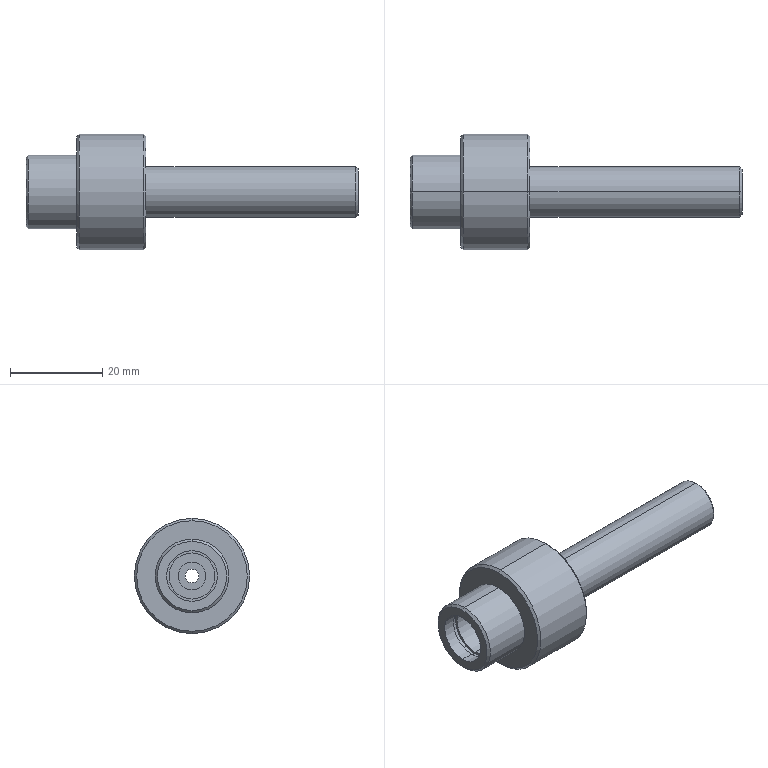Part | SolidWorks | features ICE 9, Chamfer 1, Extrusion 1, HoleWzd 1 | 1 solid | 41 faces | box 72 x 25 x 25 mm | volume 11483 mm3 | cylinder 22 | plane 11 | cone 8 | commonest cylinder face diameters 11 x6 3 x2 5.5 x2 6 x2 6.8 x2 10 x2
STEP:
#1=CARTESIAN_POINT('',(0.,0.,7.5));
#2=VERTEX_POINT('',#1);
#3=CARTESIAN_POINT('',(0.,0.,-7.5));
#4=VERTEX_POINT('',#3);
#5=CARTESIAN_POINT('',(0.,0.,0.));
#6=DIRECTION('',(-1.,0.,0.));
#7=DIRECTION('',(0.,0.,-1.));
#8=AXIS2_PLACEMENT_3D('',#5,#6,#7);
#9=CIRCLE('',#8,7.5);
#10=EDGE_CURVE('',#2,#4,#9,.T.);
#11=ORIENTED_EDGE('',*,*,#10,.F.);
#12=CARTESIAN_POINT('',(0.5,0.,8.));
#13=VERTEX_POINT('',#12);
#14=CARTESIAN_POINT('',(0.5,0.,8.));
#15=DIRECTION('',(0.7071,0.,0.7071));
#16=VECTOR('',#15,1000.);
#17=LINE('',#14,#16);
#18=EDGE_CURVE('',#2,#13,#17,.T.);
#19=ORIENTED_EDGE('',*,*,#18,.T.);
#20=CARTESIAN_POINT('',(0.5,0.,-8.));
#21=VERTEX_POINT('',#20);
#22=CARTESIAN_POINT('',(0.5,0.,0.));
#23=DIRECTION('',(1.,0.,0.));
#24=DIRECTION('',(0.,0.,-1.));
#25=AXIS2_PLACEMENT_3D('',#22,#23,#24);
#26=CIRCLE('',#25,8.);
#27=EDGE_CURVE('',#21,#13,#26,.T.);
#28=ORIENTED_EDGE('',*,*,#27,.F.);
#29=CARTESIAN_POINT('',(0.5,0.,-8.));
#30=DIRECTION('',(0.7071,0.,-0.7071));
#31=VECTOR('',#30,1000.);
#32=LINE('',#29,#31);
#33=EDGE_CURVE('',#4,#21,#32,.T.);
#34=ORIENTED_EDGE('',*,*,#33,.F.);
#35=EDGE_LOOP('',(#11,#19,#28,#34));
#36=FACE_OUTER_BOUND('',#35,.T.);
#37=CARTESIAN_POINT('',(0.5,0.,0.));
#38=DIRECTION('',(1.,0.,0.));
#39=DIRECTION('',(0.,0.,-1.));
#40=AXIS2_PLACEMENT_3D('',#37,#38,#39);
#41=CONICAL_SURFACE('',#40,8.,0.7854);
#42=ADVANCED_FACE('',(#36),#41,.T.);
#43=CARTESIAN_POINT('',(11.,0.,12.));
#44=VERTEX_POINT('',#43);
#45=CARTESIAN_POINT('',(11.,0.,-12.));
#46=VERTEX_POINT('',#45);
#47=CARTESIAN_POINT('',(11.,0.,0.));
#48=DIRECTION('',(-1.,0.,0.));
#49=DIRECTION('',(0.,0.,-1.));
#50=AXIS2_PLACEMENT_3D('',#47,#48,#49);
#51=CIRCLE('',#50,12.);
#52=EDGE_CURVE('',#44,#46,#51,.T.);
#53=ORIENTED_EDGE('',*,*,#52,.F.);
#54=CARTESIAN_POINT('',(11.5,0.,12.5));
#55=VERTEX_POINT('',#54);
#56=CARTESIAN_POINT('',(11.5,0.,12.5));
#57=DIRECTION('',(0.7071,0.,0.7071));
#58=VECTOR('',#57,1000.);
#59=LINE('',#56,#58);
#60=EDGE_CURVE('',#44,#55,#59,.T.);
#61=ORIENTED_EDGE('',*,*,#60,.T.);
#62=CARTESIAN_POINT('',(11.5,0.,-12.5));
#63=VERTEX_POINT('',#62);
#64=CARTESIAN_POINT('',(11.5,0.,0.));
#65=DIRECTION('',(1.,0.,0.));
#66=DIRECTION('',(0.,0.,-1.));
#67=AXIS2_PLACEMENT_3D('',#64,#65,#66);
#68=CIRCLE('',#67,12.5);
#69=EDGE_CURVE('',#63,#55,#68,.T.);
#70=ORIENTED_EDGE('',*,*,#69,.F.);
#71=CARTESIAN_POINT('',(11.5,0.,-12.5));
#72=DIRECTION('',(0.7071,0.,-0.7071));
#73=VECTOR('',#72,1000.);
#74=LINE('',#71,#73);
#75=EDGE_CURVE('',#46,#63,#74,.T.);
#76=ORIENTED_EDGE('',*,*,#75,.F.);
#77=EDGE_LOOP('',(#53,#61,#70,#76));
#78=FACE_OUTER_BOUND('',#77,.T.);
#79=CARTESIAN_POINT('',(11.5,0.,0.));
#80=DIRECTION('',(1.,0.,0.));
#81=DIRECTION('',(0.,0.,-1.));
#82=AXIS2_PLACEMENT_3D('',#79,#80,#81);
#83=CONICAL_SURFACE('',#82,12.5,0.7854);
#84=ADVANCED_FACE('',(#78),#83,.T.);
#85=CARTESIAN_POINT('',(26.,0.,-12.));
#86=VERTEX_POINT('',#85);
#87=CARTESIAN_POINT('',(26.,0.,12.));
#88=VERTEX_POINT('',#87);
#89=CARTESIAN_POINT('',(26.,0.,0.));
#90=DIRECTION('',(1.,0.,0.));
#91=DIRECTION('',(0.,0.,-1.));
#92=AXIS2_PLACEMENT_3D('',#89,#90,#91);
#93=CIRCLE('',#92,12.);
#94=EDGE_CURVE('',#86,#88,#93,.T.);
#95=ORIENTED_EDGE('',*,*,#94,.F.);
#96=CARTESIAN_POINT('',(25.5,0.,-12.5));
#97=VERTEX_POINT('',#96);
#98=CARTESIAN_POINT('',(26.,0.,-12.));
#99=DIRECTION('',(-0.7071,0.,-0.7071));
#100=VECTOR('',#99,1000.);
#101=LINE('',#98,#100);
#102=EDGE_CURVE('',#86,#97,#101,.T.);
#103=ORIENTED_EDGE('',*,*,#102,.T.);
#104=CARTESIAN_POINT('',(25.5,0.,12.5));
#105=VERTEX_POINT('',#104);
#106=CARTESIAN_POINT('',(25.5,0.,0.));
#107=DIRECTION('',(-1.,0.,0.));
#108=DIRECTION('',(0.,0.,-1.));
#109=AXIS2_PLACEMENT_3D('',#106,#107,#108);
#110=CIRCLE('',#109,12.5);
#111=EDGE_CURVE('',#105,#97,#110,.T.);
#112=ORIENTED_EDGE('',*,*,#111,.F.);
#113=CARTESIAN_POINT('',(26.,0.,12.));
#114=DIRECTION('',(-0.7071,0.,0.7071));
#115=VECTOR('',#114,1000.);
#116=LINE('',#113,#115);
#117=EDGE_CURVE('',#88,#105,#116,.T.);
#118=ORIENTED_EDGE('',*,*,#117,.F.);
#119=EDGE_LOOP('',(#95,#103,#112,#118));
#120=FACE_OUTER_BOUND('',#119,.T.);
#121=CARTESIAN_POINT('',(26.,0.,0.));
#122=DIRECTION('',(-1.,0.,0.));
#123=DIRECTION('',(0.,0.,1.));
#124=AXIS2_PLACEMENT_3D('',#121,#122,#123);
#125=CONICAL_SURFACE('',#124,12.,0.7854);
#126=ADVANCED_FACE('',(#120),#125,.T.);
#127=CARTESIAN_POINT('',(72.,0.,-5.));
#128=VERTEX_POINT('',#127);
#129=CARTESIAN_POINT('',(72.,0.,5.));
#130=VERTEX_POINT('',#129);
#131=CARTESIAN_POINT('',(72.,0.,0.));
#132=DIRECTION('',(1.,0.,0.));
#133=DIRECTION('',(0.,0.,-1.));
#134=AXIS2_PLACEMENT_3D('',#131,#132,#133);
#135=CIRCLE('',#134,5.);
#136=EDGE_CURVE('',#128,#130,#135,.T.);
#137=ORIENTED_EDGE('',*,*,#136,.F.);
#138=CARTESIAN_POINT('',(71.5,0.,-5.5));
#139=VERTEX_POINT('',#138);
#140=CARTESIAN_POINT('',(72.,0.,-5.));
#141=DIRECTION('',(-0.7071,0.,-0.7071));
#142=VECTOR('',#141,1000.);
#143=LINE('',#140,#142);
#144=EDGE_CURVE('',#128,#139,#143,.T.);
#145=ORIENTED_EDGE('',*,*,#144,.T.);
#146=CARTESIAN_POINT('',(71.5,0.,5.5));
#147=VERTEX_POINT('',#146);
#148=CARTESIAN_POINT('',(71.5,0.,0.));
#149=DIRECTION('',(-1.,0.,0.));
#150=DIRECTION('',(0.,0.,-1.));
#151=AXIS2_PLACEMENT_3D('',#148,#149,#150);
#152=CIRCLE('',#151,5.5);
#153=EDGE_CURVE('',#147,#139,#152,.T.);
#154=ORIENTED_EDGE('',*,*,#153,.F.);
#155=CARTESIAN_POINT('',(72.,0.,5.));
#156=DIRECTION('',(-0.7071,0.,0.7071));
#157=VECTOR('',#156,1000.);
#158=LINE('',#155,#157);
#159=EDGE_CURVE('',#130,#147,#158,.T.);
#160=ORIENTED_EDGE('',*,*,#159,.F.);
#161=EDGE_LOOP('',(#137,#145,#154,#160));
#162=FACE_OUTER_BOUND('',#161,.T.);
#163=CARTESIAN_POINT('',(72.,0.,0.));
#164=DIRECTION('',(-1.,0.,0.));
#165=DIRECTION('',(0.,0.,1.));
#166=AXIS2_PLACEMENT_3D('',#163,#164,#165);
#167=CONICAL_SURFACE('',#166,5.,0.7854);
#168=ADVANCED_FACE('',(#162),#167,.T.);
#169=CARTESIAN_POINT('',(29.,0.,-1.5));
#170=VERTEX_POINT('',#169);
#171=CARTESIAN_POINT('',(29.,0.,1.5));
#172=VERTEX_POINT('',#171);
#173=CARTESIAN_POINT('',(29.,0.,0.));
#174=DIRECTION('',(-1.,0.,0.));
#175=DIRECTION('',(0.,0.,1.));
#176=AXIS2_PLACEMENT_3D('',#173,#174,#175);
#177=CIRCLE('',#176,1.5);
#178=EDGE_CURVE('',#170,#172,#177,.T.);
#179=ORIENTED_EDGE('',*,*,#178,.T.);
#180=CARTESIAN_POINT('',(56.,0.,1.5));
#181=VERTEX_POINT('',#180);
#182=CARTESIAN_POINT('',(-32.,0.,1.5));
#183=DIRECTION('',(1.,0.,0.));
#184=VECTOR('',#183,1000.);
#185=LINE('',#182,#184);
#186=EDGE_CURVE('',#172,#181,#185,.T.);
#187=ORIENTED_EDGE('',*,*,#186,.T.);
#188=CARTESIAN_POINT('',(56.,0.,-1.5));
#189=VERTEX_POINT('',#188);
#190=CARTESIAN_POINT('',(56.,0.,0.));
#191=DIRECTION('',(1.,0.,0.));
#192=DIRECTION('',(0.,0.,-1.));
#193=AXIS2_PLACEMENT_3D('',#190,#191,#192);
#194=CIRCLE('',#193,1.5);
#195=EDGE_CURVE('',#181,#189,#194,.T.);
#196=ORIENTED_EDGE('',*,*,#195,.T.);
#197=CARTESIAN_POINT('',(-32.,0.,-1.5));
#198=DIRECTION('',(1.,0.,0.));
#199=VECTOR('',#198,1000.);
#200=LINE('',#197,#199);
#201=EDGE_CURVE('',#170,#189,#200,.T.);
#202=ORIENTED_EDGE('',*,*,#201,.F.);
#203=EDGE_LOOP('',(#179,#187,#196,#202));
#204=FACE_OUTER_BOUND('',#203,.T.);
#205=CARTESIAN_POINT('',(-32.,0.,0.));
#206=DIRECTION('',(1.,0.,0.));
#207=DIRECTION('',(0.,0.,-1.));
#208=AXIS2_PLACEMENT_3D('',#205,#206,#207);
#209=CYLINDRICAL_SURFACE('',#208,1.5);
#210=ADVANCED_FACE('',(#204),#209,.F.);
#211=CARTESIAN_POINT('',(56.,0.,2.75));
#212=VERTEX_POINT('',#211);
#213=CARTESIAN_POINT('',(56.,0.,-2.75));
#214=VERTEX_POINT('',#213);
#215=CARTESIAN_POINT('',(56.,0.,0.));
#216=DIRECTION('',(1.,0.,0.));
#217=DIRECTION('',(0.,0.,-1.));
#218=AXIS2_PLACEMENT_3D('',#215,#216,#217);
#219=CIRCLE('',#218,2.75);
#220=EDGE_CURVE('',#212,#214,#219,.T.);
#221=ORIENTED_EDGE('',*,*,#220,.F.);
#222=CARTESIAN_POINT('',(61.,0.,2.75));
#223=VERTEX_POINT('',#222);
#224=CARTESIAN_POINT('',(56.,0.,2.75));
#225=DIRECTION('',(1.,0.,0.));
#226=VECTOR('',#225,1000.);
#227=LINE('',#224,#226);
#228=EDGE_CURVE('',#212,#223,#227,.T.);
#229=ORIENTED_EDGE('',*,*,#228,.T.);
#230=CARTESIAN_POINT('',(61.,0.,-2.75));
#231=VERTEX_POINT('',#230);
#232=CARTESIAN_POINT('',(61.,0.,0.));
#233=DIRECTION('',(1.,0.,0.));
#234=DIRECTION('',(0.,0.,-1.));
#235=AXIS2_PLACEMENT_3D('',#232,#233,#234);
#236=CIRCLE('',#235,2.75);
#237=EDGE_CURVE('',#223,#231,#236,.T.);
#238=ORIENTED_EDGE('',*,*,#237,.T.);
#239=CARTESIAN_POINT('',(56.,0.,-2.75));
#240=DIRECTION('',(1.,0.,0.));
#241=VECTOR('',#240,1000.);
#242=LINE('',#239,#241);
#243=EDGE_CURVE('',#214,#231,#242,.T.);
#244=ORIENTED_EDGE('',*,*,#243,.F.);
#245=EDGE_LOOP('',(#221,#229,#238,#244));
#246=FACE_OUTER_BOUND('',#245,.T.);
#247=CARTESIAN_POINT('',(56.,0.,0.));
#248=DIRECTION('',(1.,0.,0.));
#249=DIRECTION('',(0.,0.,-1.));
#250=AXIS2_PLACEMENT_3D('',#247,#248,#249);
#251=CYLINDRICAL_SURFACE('',#250,2.75);
#252=ADVANCED_FACE('',(#246),#251,.F.);
#253=CARTESIAN_POINT('',(61.,0.,3.4));
#254=VERTEX_POINT('',#253);
#255=CARTESIAN_POINT('',(61.,0.,-3.4));
#256=VERTEX_POINT('',#255);
#257=CARTESIAN_POINT('',(61.,0.,0.));
#258=DIRECTION('',(1.,0.,0.));
#259=DIRECTION('',(0.,0.,-1.));
#260=AXIS2_PLACEMENT_3D('',#257,#258,#259);
#261=CIRCLE('',#260,3.4);
#262=EDGE_CURVE('',#254,#256,#261,.T.);
#263=ORIENTED_EDGE('',*,*,#262,.F.);
#264=CARTESIAN_POINT('',(72.,0.,3.4));
#265=VERTEX_POINT('',#264);
#266=CARTESIAN_POINT('',(72.,0.,3.4));
#267=DIRECTION('',(1.,0.,0.));
#268=VECTOR('',#267,1000.);
#269=LINE('',#266,#268);
#270=EDGE_CURVE('',#254,#265,#269,.T.);
#271=ORIENTED_EDGE('',*,*,#270,.T.);
#272=CARTESIAN_POINT('',(72.,0.,-3.4));
#273=VERTEX_POINT('',#272);
#274=CARTESIAN_POINT('',(72.,0.,0.));
#275=DIRECTION('',(1.,0.,0.));
#276=DIRECTION('',(0.,0.,-1.));
#277=AXIS2_PLACEMENT_3D('',#274,#275,#276);
#278=CIRCLE('',#277,3.4);
#279=EDGE_CURVE('',#265,#273,#278,.T.);
#280=ORIENTED_EDGE('',*,*,#279,.T.);
#281=CARTESIAN_POINT('',(72.,0.,-3.4));
#282=DIRECTION('',(1.,0.,0.));
#283=VECTOR('',#282,1000.);
#284=LINE('',#281,#283);
#285=EDGE_CURVE('',#256,#273,#284,.T.);
#286=ORIENTED_EDGE('',*,*,#285,.F.);
#287=EDGE_LOOP('',(#263,#271,#280,#286));
#288=FACE_OUTER_BOUND('',#287,.T.);
#289=CARTESIAN_POINT('',(72.,0.,0.));
#290=DIRECTION('',(1.,0.,0.));
#291=DIRECTION('',(0.,0.,-1.));
#292=AXIS2_PLACEMENT_3D('',#289,#290,#291);
#293=CYLINDRICAL_SURFACE('',#292,3.4);
#294=ADVANCED_FACE('',(#288),#293,.F.);
#295=CARTESIAN_POINT('',(29.,0.,-3.));
#296=VERTEX_POINT('',#295);
#297=CARTESIAN_POINT('',(29.,0.,3.));
#298=VERTEX_POINT('',#297);
#299=CARTESIAN_POINT('',(29.,0.,0.));
#300=DIRECTION('',(-1.,0.,0.));
#301=DIRECTION('',(0.,0.,1.));
#302=AXIS2_PLACEMENT_3D('',#299,#300,#301);
#303=CIRCLE('',#302,3.);
#304=EDGE_CURVE('',#296,#298,#303,.T.);
#305=ORIENTED_EDGE('',*,*,#304,.F.);
#306=CARTESIAN_POINT('',(14.,0.,-3.));
#307=VERTEX_POINT('',#306);
#308=CARTESIAN_POINT('',(29.,0.,-3.));
#309=DIRECTION('',(-1.,0.,0.));
#310=VECTOR('',#309,1000.);
#311=LINE('',#308,#310);
#312=EDGE_CURVE('',#296,#307,#311,.T.);
#313=ORIENTED_EDGE('',*,*,#312,.T.);
#314=CARTESIAN_POINT('',(14.,0.,3.));
#315=VERTEX_POINT('',#314);
#316=CARTESIAN_POINT('',(14.,0.,0.));
#317=DIRECTION('',(-1.,0.,0.));
#318=DIRECTION('',(0.,0.,1.));
#319=AXIS2_PLACEMENT_3D('',#316,#317,#318);
#320=CIRCLE('',#319,3.);
#321=EDGE_CURVE('',#307,#315,#320,.T.);
#322=ORIENTED_EDGE('',*,*,#321,.T.);
#323=CARTESIAN_POINT('',(29.,0.,3.));
#324=DIRECTION('',(-1.,0.,0.));
#325=VECTOR('',#324,1000.);
#326=LINE('',#323,#325);
#327=EDGE_CURVE('',#298,#315,#326,.T.);
#328=ORIENTED_EDGE('',*,*,#327,.F.);
#329=EDGE_LOOP('',(#305,#313,#322,#328));
#330=FACE_OUTER_BOUND('',#329,.T.);
#331=CARTESIAN_POINT('',(29.,0.,0.));
#332=DIRECTION('',(-1.,0.,0.));
#333=DIRECTION('',(0.,0.,1.));
#334=AXIS2_PLACEMENT_3D('',#331,#332,#333);
#335=CYLINDRICAL_SURFACE('',#334,3.);
#336=ADVANCED_FACE('',(#330),#335,.F.);
#337=CARTESIAN_POINT('',(14.,0.,-5.));
#338=VERTEX_POINT('',#337);
#339=CARTESIAN_POINT('',(14.,0.,5.));
#340=VERTEX_POINT('',#339);
#341=CARTESIAN_POINT('',(14.,0.,0.));
#342=DIRECTION('',(-1.,0.,0.));
#343=DIRECTION('',(0.,0.,1.));
#344=AXIS2_PLACEMENT_3D('',#341,#342,#343);
#345=CIRCLE('',#344,5.);
#346=EDGE_CURVE('',#338,#340,#345,.T.);
#347=ORIENTED_EDGE('',*,*,#346,.F.);
#348=CARTESIAN_POINT('',(11.,0.,-5.));
#349=VERTEX_POINT('',#348);
#350=CARTESIAN_POINT('',(14.,0.,-5.));
#351=DIRECTION('',(-1.,0.,0.));
#352=VECTOR('',#351,1000.);
#353=LINE('',#350,#352);
#354=EDGE_CURVE('',#338,#349,#353,.T.);
#355=ORIENTED_EDGE('',*,*,#354,.T.);
#356=CARTESIAN_POINT('',(11.,0.,5.));
#357=VERTEX_POINT('',#356);
#358=CARTESIAN_POINT('',(11.,0.,0.));
#359=DIRECTION('',(-1.,0.,0.));
#360=DIRECTION('',(0.,0.,1.));
#361=AXIS2_PLACEMENT_3D('',#358,#359,#360);
#362=CIRCLE('',#361,5.);
#363=EDGE_CURVE('',#349,#357,#362,.T.);
#364=ORIENTED_EDGE('',*,*,#363,.T.);
#365=CARTESIAN_POINT('',(14.,0.,5.));
#366=DIRECTION('',(-1.,0.,0.));
#367=VECTOR('',#366,1000.);
#368=LINE('',#365,#367);
#369=EDGE_CURVE('',#340,#357,#368,.T.);
#370=ORIENTED_EDGE('',*,*,#369,.F.);
#371=EDGE_LOOP('',(#347,#355,#364,#370));
#372=FACE_OUTER_BOUND('',#371,.T.);
#373=CARTESIAN_POINT('',(14.,0.,0.));
#374=DIRECTION('',(-1.,0.,0.));
#375=DIRECTION('',(0.,0.,1.));
#376=AXIS2_PLACEMENT_3D('',#373,#374,#375);
#377=CYLINDRICAL_SURFACE('',#376,5.);
#378=ADVANCED_FACE('',(#372),#377,.F.);
#379=CARTESIAN_POINT('',(11.,0.,-5.5));
#380=VERTEX_POINT('',#379);
#381=CARTESIAN_POINT('',(11.,0.,5.5));
#382=VERTEX_POINT('',#381);
#383=CARTESIAN_POINT('',(11.,0.,0.));
#384=DIRECTION('',(-1.,0.,0.));
#385=DIRECTION('',(0.,0.,1.));
#386=AXIS2_PLACEMENT_3D('',#383,#384,#385);
#387=CIRCLE('',#386,5.5);
#388=EDGE_CURVE('',#380,#382,#387,.T.);
#389=ORIENTED_EDGE('',*,*,#388,.F.);
#390=CARTESIAN_POINT('',(3.8,0.,-5.5));
#391=VERTEX_POINT('',#390);
#392=CARTESIAN_POINT('',(11.,0.,-5.5));
#393=DIRECTION('',(-1.,0.,0.));
#394=VECTOR('',#393,1000.);
#395=LINE('',#392,#394);
#396=EDGE_CURVE('',#380,#391,#395,.T.);
#397=ORIENTED_EDGE('',*,*,#396,.T.);
#398=CARTESIAN_POINT('',(3.8,0.,5.5));
#399=VERTEX_POINT('',#398);
#400=CARTESIAN_POINT('',(3.8,0.,0.));
#401=DIRECTION('',(1.,0.,0.));
#402=DIRECTION('',(0.,0.,1.));
#403=AXIS2_PLACEMENT_3D('',#400,#401,#402);
#404=CIRCLE('',#403,5.5);
#405=EDGE_CURVE('',#399,#391,#404,.T.);
#406=ORIENTED_EDGE('',*,*,#405,.F.);
#407=CARTESIAN_POINT('',(11.,0.,5.5));
#408=DIRECTION('',(-1.,0.,0.));
#409=VECTOR('',#408,1000.);
#410=LINE('',#407,#409);
#411=EDGE_CURVE('',#382,#399,#410,.T.);
#412=ORIENTED_EDGE('',*,*,#411,.F.);
#413=EDGE_LOOP('',(#389,#397,#406,#412));
#414=FACE_OUTER_BOUND('',#413,.T.);
#415=CARTESIAN_POINT('',(11.,0.,0.));
#416=DIRECTION('',(-1.,0.,0.));
#417=DIRECTION('',(0.,0.,1.));
#418=AXIS2_PLACEMENT_3D('',#415,#416,#417);
#419=CYLINDRICAL_SURFACE('',#418,5.5);
#420=ADVANCED_FACE('',(#414),#419,.F.);
#421=CARTESIAN_POINT('',(3.8,0.,-6.));
#422=VERTEX_POINT('',#421);
#423=CARTESIAN_POINT('',(3.8,0.,6.));
#424=VERTEX_POINT('',#423);
#425=CARTESIAN_POINT('',(3.8,0.,0.));
#426=DIRECTION('',(-1.,0.,0.));
#427=DIRECTION('',(0.,0.,1.));
#428=AXIS2_PLACEMENT_3D('',#425,#426,#427);
#429=CIRCLE('',#428,6.);
#430=EDGE_CURVE('',#422,#424,#429,.T.);
#431=ORIENTED_EDGE('',*,*,#430,.F.);
#432=CARTESIAN_POINT('',(2.7,0.,-6.));
#433=VERTEX_POINT('',#432);
#434=CARTESIAN_POINT('',(3.8,0.,-6.));
#435=DIRECTION('',(-1.,0.,0.));
#436=VECTOR('',#435,1000.);
#437=LINE('',#434,#436);
#438=EDGE_CURVE('',#422,#433,#437,.T.);
#439=ORIENTED_EDGE('',*,*,#438,.T.);
#440=CARTESIAN_POINT('',(2.7,0.,6.));
#441=VERTEX_POINT('',#440);
#442=CARTESIAN_POINT('',(2.7,0.,0.));
#443=DIRECTION('',(-1.,0.,0.));
#444=DIRECTION('',(0.,0.,1.));
#445=AXIS2_PLACEMENT_3D('',#442,#443,#444);
#446=CIRCLE('',#445,6.);
#447=EDGE_CURVE('',#433,#441,#446,.T.);
#448=ORIENTED_EDGE('',*,*,#447,.T.);
#449=CARTESIAN_POINT('',(3.8,0.,6.));
#450=DIRECTION('',(-1.,0.,0.));
#451=VECTOR('',#450,1000.);
#452=LINE('',#449,#451);
#453=EDGE_CURVE('',#424,#441,#452,.T.);
#454=ORIENTED_EDGE('',*,*,#453,.F.);
#455=EDGE_LOOP('',(#431,#439,#448,#454));
#456=FACE_OUTER_BOUND('',#455,.T.);
#457=CARTESIAN_POINT('',(3.8,0.,0.));
#458=DIRECTION('',(-1.,0.,0.));
#459=DIRECTION('',(0.,0.,1.));
#460=AXIS2_PLACEMENT_3D('',#457,#458,#459);
#461=CYLINDRICAL_SURFACE('',#460,6.);
#462=ADVANCED_FACE('',(#456),#461,.F.);
#463=CARTESIAN_POINT('',(2.7,0.,5.5));
#464=VERTEX_POINT('',#463);
#465=CARTESIAN_POINT('',(2.7,0.,-5.5));
#466=VERTEX_POINT('',#465);
#467=CARTESIAN_POINT('',(2.7,0.,0.));
#468=DIRECTION('',(1.,0.,0.));
#469=DIRECTION('',(0.,0.,1.));
#470=AXIS2_PLACEMENT_3D('',#467,#468,#469);
#471=CIRCLE('',#470,5.5);
#472=EDGE_CURVE('',#464,#466,#471,.T.);
#473=ORIENTED_EDGE('',*,*,#472,.T.);
#474=CARTESIAN_POINT('',(0.,0.,-5.5));
#475=VERTEX_POINT('',#474);
#476=CARTESIAN_POINT('',(11.,0.,-5.5));
#477=DIRECTION('',(-1.,0.,0.));
#478=VECTOR('',#477,1000.);
#479=LINE('',#476,#478);
#480=EDGE_CURVE('',#466,#475,#479,.T.);
#481=ORIENTED_EDGE('',*,*,#480,.T.);
#482=CARTESIAN_POINT('',(0.,0.,5.5));
#483=VERTEX_POINT('',#482);
#484=CARTESIAN_POINT('',(0.,0.,0.));
#485=DIRECTION('',(-1.,0.,0.));
#486=DIRECTION('',(0.,0.,1.));
#487=AXIS2_PLACEMENT_3D('',#484,#485,#486);
#488=CIRCLE('',#487,5.5);
#489=EDGE_CURVE('',#475,#483,#488,.T.);
#490=ORIENTED_EDGE('',*,*,#489,.T.);
#491=CARTESIAN_POINT('',(11.,0.,5.5));
#492=DIRECTION('',(-1.,0.,0.));
#493=VECTOR('',#492,1000.);
#494=LINE('',#491,#493);
#495=EDGE_CURVE('',#464,#483,#494,.T.);
#496=ORIENTED_EDGE('',*,*,#495,.F.);
#497=EDGE_LOOP('',(#473,#481,#490,#496));
#498=FACE_OUTER_BOUND('',#497,.T.);
#499=CARTESIAN_POINT('',(11.,0.,0.));
#500=DIRECTION('',(-1.,0.,0.));
#501=DIRECTION('',(0.,0.,1.));
#502=AXIS2_PLACEMENT_3D('',#499,#500,#501);
#503=CYLINDRICAL_SURFACE('',#502,5.5);
#504=ADVANCED_FACE('',(#498),#503,.F.);
#505=ORIENTED_EDGE('',*,*,#153,.T.);
#506=CARTESIAN_POINT('',(26.,0.,-5.5));
#507=VERTEX_POINT('',#506);
#508=CARTESIAN_POINT('',(72.,0.,-5.5));
#509=DIRECTION('',(-1.,0.,0.));
#510=VECTOR('',#509,1000.);
#511=LINE('',#508,#510);
#512=EDGE_CURVE('',#139,#507,#511,.T.);
#513=ORIENTED_EDGE('',*,*,#512,.T.);
#514=CARTESIAN_POINT('',(26.,0.,5.5));
#515=VERTEX_POINT('',#514);
#516=CARTESIAN_POINT('',(26.,0.,0.));
#517=DIRECTION('',(1.,0.,0.));
#518=DIRECTION('',(0.,0.,-1.));
#519=AXIS2_PLACEMENT_3D('',#516,#517,#518);
#520=CIRCLE('',#519,5.5);
#521=EDGE_CURVE('',#507,#515,#520,.T.);
#522=ORIENTED_EDGE('',*,*,#521,.T.);
#523=CARTESIAN_POINT('',(72.,0.,5.5));
#524=DIRECTION('',(-1.,0.,0.));
#525=VECTOR('',#524,1000.);
#526=LINE('',#523,#525);
#527=EDGE_CURVE('',#147,#515,#526,.T.);
#528=ORIENTED_EDGE('',*,*,#527,.F.);
#529=EDGE_LOOP('',(#505,#513,#522,#528));
#530=FACE_OUTER_BOUND('',#529,.T.);
#531=CARTESIAN_POINT('',(72.,0.,0.));
#532=DIRECTION('',(-1.,0.,0.));
#533=DIRECTION('',(0.,0.,1.));
#534=AXIS2_PLACEMENT_3D('',#531,#532,#533);
#535=CYLINDRICAL_SURFACE('',#534,5.5);
#536=ADVANCED_FACE('',(#530),#535,.T.);
#537=ORIENTED_EDGE('',*,*,#111,.T.);
#538=CARTESIAN_POINT('',(26.,0.,-12.5));
#539=DIRECTION('',(-1.,0.,0.));
#540=VECTOR('',#539,1000.);
#541=LINE('',#538,#540);
#542=EDGE_CURVE('',#97,#63,#541,.T.);
#543=ORIENTED_EDGE('',*,*,#542,.T.);
#544=ORIENTED_EDGE('',*,*,#69,.T.);
#545=CARTESIAN_POINT('',(26.,0.,12.5));
#546=DIRECTION('',(-1.,0.,0.));
#547=VECTOR('',#546,1000.);
#548=LINE('',#545,#547);
#549=EDGE_CURVE('',#105,#55,#548,.T.);
#550=ORIENTED_EDGE('',*,*,#549,.F.);
#551=EDGE_LOOP('',(#537,#543,#544,#550));
#552=FACE_OUTER_BOUND('',#551,.T.);
#553=CARTESIAN_POINT('',(26.,0.,0.));
#554=DIRECTION('',(-1.,0.,0.));
#555=DIRECTION('',(0.,0.,1.));
#556=AXIS2_PLACEMENT_3D('',#553,#554,#555);
#557=CYLINDRICAL_SURFACE('',#556,12.5);
#558=ADVANCED_FACE('',(#552),#557,.T.);
#559=CARTESIAN_POINT('',(11.,0.,-8.));
#560=VERTEX_POINT('',#559);
#561=CARTESIAN_POINT('',(11.,0.,8.));
#562=VERTEX_POINT('',#561);
#563=CARTESIAN_POINT('',(11.,0.,0.));
#564=DIRECTION('',(1.,0.,0.));
#565=DIRECTION('',(0.,0.,-1.));
#566=AXIS2_PLACEMENT_3D('',#563,#564,#565);
#567=CIRCLE('',#566,8.);
#568=EDGE_CURVE('',#560,#562,#567,.T.);
#569=ORIENTED_EDGE('',*,*,#568,.F.);
#570=CARTESIAN_POINT('',(11.,0.,-8.));
#571=DIRECTION('',(-1.,0.,0.));
#572=VECTOR('',#571,1000.);
#573=LINE('',#570,#572);
#574=EDGE_CURVE('',#560,#21,#573,.T.);
#575=ORIENTED_EDGE('',*,*,#574,.T.);
#576=ORIENTED_EDGE('',*,*,#27,.T.);
#577=CARTESIAN_POINT('',(11.,0.,8.));
#578=DIRECTION('',(-1.,0.,0.));
#579=VECTOR('',#578,1000.);
#580=LINE('',#577,#579);
#581=EDGE_CURVE('',#562,#13,#580,.T.);
#582=ORIENTED_EDGE('',*,*,#581,.F.);
#583=EDGE_LOOP('',(#569,#575,#576,#582));
#584=FACE_OUTER_BOUND('',#583,.T.);
#585=CARTESIAN_POINT('',(11.,0.,0.));
#586=DIRECTION('',(-1.,0.,0.));
#587=DIRECTION('',(0.,0.,1.));
#588=AXIS2_PLACEMENT_3D('',#585,#586,#587);
#589=CYLINDRICAL_SURFACE('',#588,8.);
#590=ADVANCED_FACE('',(#584),#589,.T.);
#591=ORIENTED_EDGE('',*,*,#574,.F.);
#592=CARTESIAN_POINT('',(11.,0.,0.));
#593=DIRECTION('',(1.,0.,0.));
#594=DIRECTION('',(0.,0.,-1.));
#595=AXIS2_PLACEMENT_3D('',#592,#593,#594);
#596=CIRCLE('',#595,8.);
#597=EDGE_CURVE('',#562,#560,#596,.T.);
#598=ORIENTED_EDGE('',*,*,#597,.F.);
#599=ORIENTED_EDGE('',*,*,#581,.T.);
#600=CARTESIAN_POINT('',(0.5,0.,0.));
#601=DIRECTION('',(1.,0.,0.));
#602=DIRECTION('',(0.,0.,-1.));
#603=AXIS2_PLACEMENT_3D('',#600,#601,#602);
#604=CIRCLE('',#603,8.);
#605=EDGE_CURVE('',#13,#21,#604,.T.);
#606=ORIENTED_EDGE('',*,*,#605,.T.);
#607=EDGE_LOOP('',(#591,#598,#599,#606));
#608=FACE_OUTER_BOUND('',#607,.T.);
#609=CARTESIAN_POINT('',(11.,0.,0.));
#610=DIRECTION('',(-1.,0.,0.));
#611=DIRECTION('',(0.,0.,1.));
#612=AXIS2_PLACEMENT_3D('',#609,#610,#611);
#613=CYLINDRICAL_SURFACE('',#612,8.);
#614=ADVANCED_FACE('',(#608),#613,.T.);
#615=CARTESIAN_POINT('',(0.,0.,0.));
#616=DIRECTION('',(-1.,0.,0.));
#617=DIRECTION('',(0.,0.,-1.));
#618=AXIS2_PLACEMENT_3D('',#615,#616,#617);
#619=CIRCLE('',#618,7.5);
#620=EDGE_CURVE('',#4,#2,#619,.T.);
#621=ORIENTED_EDGE('',*,*,#620,.T.);
#622=ORIENTED_EDGE('',*,*,#10,.T.);
#623=EDGE_LOOP('',(#621,#622));
#624=FACE_OUTER_BOUND('',#623,.T.);
#625=CARTESIAN_POINT('',(0.,0.,0.));
#626=DIRECTION('',(-1.,0.,0.));
#627=DIRECTION('',(0.,0.,1.));
#628=AXIS2_PLACEMENT_3D('',#625,#626,#627);
#629=CIRCLE('',#628,5.5);
#630=EDGE_CURVE('',#483,#475,#629,.T.);
#631=ORIENTED_EDGE('',*,*,#630,.F.);
#632=ORIENTED_EDGE('',*,*,#489,.F.);
#633=EDGE_LOOP('',(#631,#632));
#634=FACE_BOUND('',#633,.T.);
#635=CARTESIAN_POINT('',(0.,0.,0.));
#636=DIRECTION('',(1.,0.,0.));
#637=DIRECTION('',(0.,0.,-1.));
#638=AXIS2_PLACEMENT_3D('',#635,#636,#637);
#639=PLANE('',#638);
#640=ADVANCED_FACE('',(#624,#634),#639,.F.);
#641=ORIENTED_EDGE('',*,*,#542,.F.);
#642=CARTESIAN_POINT('',(25.5,0.,0.));
#643=DIRECTION('',(-1.,0.,0.));
#644=DIRECTION('',(0.,0.,-1.));
#645=AXIS2_PLACEMENT_3D('',#642,#643,#644);
#646=CIRCLE('',#645,12.5);
#647=EDGE_CURVE('',#97,#105,#646,.T.);
#648=ORIENTED_EDGE('',*,*,#647,.T.);
#649=ORIENTED_EDGE('',*,*,#549,.T.);
#650=CARTESIAN_POINT('',(11.5,0.,0.));
#651=DIRECTION('',(1.,0.,0.));
#652=DIRECTION('',(0.,0.,-1.));
#653=AXIS2_PLACEMENT_3D('',#650,#651,#652);
#654=CIRCLE('',#653,12.5);
#655=EDGE_CURVE('',#55,#63,#654,.T.);
#656=ORIENTED_EDGE('',*,*,#655,.T.);
#657=EDGE_LOOP('',(#641,#648,#649,#656));
#658=FACE_OUTER_BOUND('',#657,.T.);
#659=CARTESIAN_POINT('',(26.,0.,0.));
#660=DIRECTION('',(-1.,0.,0.));
#661=DIRECTION('',(0.,0.,1.));
#662=AXIS2_PLACEMENT_3D('',#659,#660,#661);
#663=CYLINDRICAL_SURFACE('',#662,12.5);
#664=ADVANCED_FACE('',(#658),#663,.T.);
#665=CARTESIAN_POINT('',(26.,0.,0.));
#666=DIRECTION('',(1.,0.,0.));
#667=DIRECTION('',(0.,0.,-1.));
#668=AXIS2_PLACEMENT_3D('',#665,#666,#667);
#669=CIRCLE('',#668,12.);
#670=EDGE_CURVE('',#88,#86,#669,.T.);
#671=ORIENTED_EDGE('',*,*,#670,.T.);
#672=ORIENTED_EDGE('',*,*,#94,.T.);
#673=EDGE_LOOP('',(#671,#672));
#674=FACE_OUTER_BOUND('',#673,.T.);
#675=CARTESIAN_POINT('',(26.,0.,0.));
#676=DIRECTION('',(1.,0.,0.));
#677=DIRECTION('',(0.,0.,-1.));
#678=AXIS2_PLACEMENT_3D('',#675,#676,#677);
#679=CIRCLE('',#678,5.5);
#680=EDGE_CURVE('',#515,#507,#679,.T.);
#681=ORIENTED_EDGE('',*,*,#680,.F.);
#682=ORIENTED_EDGE('',*,*,#521,.F.);
#683=EDGE_LOOP('',(#681,#682));
#684=FACE_BOUND('',#683,.T.);
#685=CARTESIAN_POINT('',(26.,0.,0.));
#686=DIRECTION('',(1.,0.,0.));
#687=DIRECTION('',(0.,0.,-1.));
#688=AXIS2_PLACEMENT_3D('',#685,#686,#687);
#689=PLANE('',#688);
#690=ADVANCED_FACE('',(#674,#684),#689,.T.);
#691=CARTESIAN_POINT('',(11.,0.,0.));
#692=DIRECTION('',(-1.,0.,0.));
#693=DIRECTION('',(0.,0.,-1.));
#694=AXIS2_PLACEMENT_3D('',#691,#692,#693);
#695=CIRCLE('',#694,12.);
#696=EDGE_CURVE('',#46,#44,#695,.T.);
#697=ORIENTED_EDGE('',*,*,#696,.T.);
#698=ORIENTED_EDGE('',*,*,#52,.T.);
#699=EDGE_LOOP('',(#697,#698));
#700=FACE_OUTER_BOUND('',#699,.T.);
#701=ORIENTED_EDGE('',*,*,#597,.T.);
#702=ORIENTED_EDGE('',*,*,#568,.T.);
#703=EDGE_LOOP('',(#701,#702));
#704=FACE_BOUND('',#703,.T.);
#705=CARTESIAN_POINT('',(11.,0.,0.));
#706=DIRECTION('',(1.,0.,0.));
#707=DIRECTION('',(0.,0.,-1.));
#708=AXIS2_PLACEMENT_3D('',#705,#706,#707);
#709=PLANE('',#708);
#710=ADVANCED_FACE('',(#700,#704),#709,.F.);
#711=ORIENTED_EDGE('',*,*,#512,.F.);
#712=CARTESIAN_POINT('',(71.5,0.,0.));
#713=DIRECTION('',(-1.,0.,0.));
#714=DIRECTION('',(0.,0.,-1.));
#715=AXIS2_PLACEMENT_3D('',#712,#713,#714);
#716=CIRCLE('',#715,5.5);
#717=EDGE_CURVE('',#139,#147,#716,.T.);
#718=ORIENTED_EDGE('',*,*,#717,.T.);
#719=ORIENTED_EDGE('',*,*,#527,.T.);
#720=ORIENTED_EDGE('',*,*,#680,.T.);
#721=EDGE_LOOP('',(#711,#718,#719,#720));
#722=FACE_OUTER_BOUND('',#721,.T.);
#723=CARTESIAN_POINT('',(72.,0.,0.));
#724=DIRECTION('',(-1.,0.,0.));
#725=DIRECTION('',(0.,0.,1.));
#726=AXIS2_PLACEMENT_3D('',#723,#724,#725);
#727=CYLINDRICAL_SURFACE('',#726,5.5);
#728=ADVANCED_FACE('',(#722),#727,.T.);
#729=CARTESIAN_POINT('',(72.,0.,0.));
#730=DIRECTION('',(1.,0.,0.));
#731=DIRECTION('',(0.,0.,-1.));
#732=AXIS2_PLACEMENT_3D('',#729,#730,#731);
#733=CIRCLE('',#732,5.);
#734=EDGE_CURVE('',#130,#128,#733,.T.);
#735=ORIENTED_EDGE('',*,*,#734,.T.);
#736=ORIENTED_EDGE('',*,*,#136,.T.);
#737=EDGE_LOOP('',(#735,#736));
#738=FACE_OUTER_BOUND('',#737,.T.);
#739=CARTESIAN_POINT('',(72.,0.,0.));
#740=DIRECTION('',(1.,0.,0.));
#741=DIRECTION('',(0.,0.,-1.));
#742=AXIS2_PLACEMENT_3D('',#739,#740,#741);
#743=CIRCLE('',#742,3.4);
#744=EDGE_CURVE('',#273,#265,#743,.T.);
#745=ORIENTED_EDGE('',*,*,#744,.F.);
#746=ORIENTED_EDGE('',*,*,#279,.F.);
#747=EDGE_LOOP('',(#745,#746));
#748=FACE_BOUND('',#747,.T.);
#749=CARTESIAN_POINT('',(72.,0.,0.));
#750=DIRECTION('',(1.,0.,0.));
#751=DIRECTION('',(0.,0.,-1.));
#752=AXIS2_PLACEMENT_3D('',#749,#750,#751);
#753=PLANE('',#752);
#754=ADVANCED_FACE('',(#738,#748),#753,.T.);
#755=ORIENTED_EDGE('',*,*,#480,.F.);
#756=CARTESIAN_POINT('',(2.7,0.,0.));
#757=DIRECTION('',(1.,0.,0.));
#758=DIRECTION('',(0.,0.,1.));
#759=AXIS2_PLACEMENT_3D('',#756,#757,#758);
#760=CIRCLE('',#759,5.5);
#761=EDGE_CURVE('',#466,#464,#760,.T.);
#762=ORIENTED_EDGE('',*,*,#761,.T.);
#763=ORIENTED_EDGE('',*,*,#495,.T.);
#764=ORIENTED_EDGE('',*,*,#630,.T.);
#765=EDGE_LOOP('',(#755,#762,#763,#764));
#766=FACE_OUTER_BOUND('',#765,.T.);
#767=CARTESIAN_POINT('',(11.,0.,0.));
#768=DIRECTION('',(-1.,0.,0.));
#769=DIRECTION('',(0.,0.,1.));
#770=AXIS2_PLACEMENT_3D('',#767,#768,#769);
#771=CYLINDRICAL_SURFACE('',#770,5.5);
#772=ADVANCED_FACE('',(#766),#771,.F.);
#773=CARTESIAN_POINT('',(3.8,0.,0.));
#774=DIRECTION('',(-1.,0.,0.));
#775=DIRECTION('',(0.,0.,1.));
#776=AXIS2_PLACEMENT_3D('',#773,#774,#775);
#777=CIRCLE('',#776,6.);
#778=EDGE_CURVE('',#424,#422,#777,.T.);
#779=ORIENTED_EDGE('',*,*,#778,.T.);
#780=ORIENTED_EDGE('',*,*,#430,.T.);
#781=EDGE_LOOP('',(#779,#780));
#782=FACE_OUTER_BOUND('',#781,.T.);
#783=ORIENTED_EDGE('',*,*,#405,.T.);
#784=CARTESIAN_POINT('',(3.8,0.,0.));
#785=DIRECTION('',(1.,0.,0.));
#786=DIRECTION('',(0.,0.,1.));
#787=AXIS2_PLACEMENT_3D('',#784,#785,#786);
#788=CIRCLE('',#787,5.5);
#789=EDGE_CURVE('',#391,#399,#788,.T.);
#790=ORIENTED_EDGE('',*,*,#789,.T.);
#791=EDGE_LOOP('',(#783,#790));
#792=FACE_BOUND('',#791,.T.);
#793=CARTESIAN_POINT('',(3.8,0.,0.));
#794=DIRECTION('',(-1.,0.,0.));
#795=DIRECTION('',(0.,0.,1.));
#796=AXIS2_PLACEMENT_3D('',#793,#794,#795);
#797=PLANE('',#796);
#798=ADVANCED_FACE('',(#782,#792),#797,.T.);
#799=CARTESIAN_POINT('',(2.7,0.,0.));
#800=DIRECTION('',(-1.,0.,0.));
#801=DIRECTION('',(0.,0.,1.));
#802=AXIS2_PLACEMENT_3D('',#799,#800,#801);
#803=CIRCLE('',#802,6.);
#804=EDGE_CURVE('',#441,#433,#803,.T.);
#805=ORIENTED_EDGE('',*,*,#804,.F.);
#806=ORIENTED_EDGE('',*,*,#447,.F.);
#807=EDGE_LOOP('',(#805,#806));
#808=FACE_OUTER_BOUND('',#807,.T.);
#809=ORIENTED_EDGE('',*,*,#472,.F.);
#810=ORIENTED_EDGE('',*,*,#761,.F.);
#811=EDGE_LOOP('',(#809,#810));
#812=FACE_BOUND('',#811,.T.);
#813=CARTESIAN_POINT('',(2.7,0.,0.));
#814=DIRECTION('',(-1.,0.,0.));
#815=DIRECTION('',(0.,0.,1.));
#816=AXIS2_PLACEMENT_3D('',#813,#814,#815);
#817=PLANE('',#816);
#818=ADVANCED_FACE('',(#808,#812),#817,.F.);
#819=ORIENTED_EDGE('',*,*,#438,.F.);
#820=ORIENTED_EDGE('',*,*,#778,.F.);
#821=ORIENTED_EDGE('',*,*,#453,.T.);
#822=ORIENTED_EDGE('',*,*,#804,.T.);
#823=EDGE_LOOP('',(#819,#820,#821,#822));
#824=FACE_OUTER_BOUND('',#823,.T.);
#825=CARTESIAN_POINT('',(3.8,0.,0.));
#826=DIRECTION('',(-1.,0.,0.));
#827=DIRECTION('',(0.,0.,1.));
#828=AXIS2_PLACEMENT_3D('',#825,#826,#827);
#829=CYLINDRICAL_SURFACE('',#828,6.);
#830=ADVANCED_FACE('',(#824),#829,.F.);
#831=CARTESIAN_POINT('',(11.,0.,0.));
#832=DIRECTION('',(-1.,0.,0.));
#833=DIRECTION('',(0.,0.,1.));
#834=AXIS2_PLACEMENT_3D('',#831,#832,#833);
#835=CIRCLE('',#834,5.);
#836=EDGE_CURVE('',#357,#349,#835,.T.);
#837=ORIENTED_EDGE('',*,*,#836,.F.);
#838=ORIENTED_EDGE('',*,*,#363,.F.);
#839=EDGE_LOOP('',(#837,#838));
#840=FACE_BOUND('',#839,.T.);
#841=CARTESIAN_POINT('',(11.,0.,0.));
#842=DIRECTION('',(-1.,0.,0.));
#843=DIRECTION('',(0.,0.,1.));
#844=AXIS2_PLACEMENT_3D('',#841,#842,#843);
#845=CIRCLE('',#844,5.5);
#846=EDGE_CURVE('',#382,#380,#845,.T.);
#847=ORIENTED_EDGE('',*,*,#846,.T.);
#848=ORIENTED_EDGE('',*,*,#388,.T.);
#849=EDGE_LOOP('',(#847,#848));
#850=FACE_OUTER_BOUND('',#849,.T.);
#851=CARTESIAN_POINT('',(11.,0.,0.));
#852=DIRECTION('',(-1.,0.,0.));
#853=DIRECTION('',(0.,0.,1.));
#854=AXIS2_PLACEMENT_3D('',#851,#852,#853);
#855=PLANE('',#854);
#856=ADVANCED_FACE('',(#840,#850),#855,.T.);
#857=ORIENTED_EDGE('',*,*,#396,.F.);
#858=ORIENTED_EDGE('',*,*,#846,.F.);
#859=ORIENTED_EDGE('',*,*,#411,.T.);
#860=ORIENTED_EDGE('',*,*,#789,.F.);
#861=EDGE_LOOP('',(#857,#858,#859,#860));
#862=FACE_OUTER_BOUND('',#861,.T.);
#863=CARTESIAN_POINT('',(11.,0.,0.));
#864=DIRECTION('',(-1.,0.,0.));
#865=DIRECTION('',(0.,0.,1.));
#866=AXIS2_PLACEMENT_3D('',#863,#864,#865);
#867=CYLINDRICAL_SURFACE('',#866,5.5);
#868=ADVANCED_FACE('',(#862),#867,.F.);
#869=ORIENTED_EDGE('',*,*,#354,.F.);
#870=CARTESIAN_POINT('',(14.,0.,0.));
#871=DIRECTION('',(-1.,0.,0.));
#872=DIRECTION('',(0.,0.,1.));
#873=AXIS2_PLACEMENT_3D('',#870,#871,#872);
#874=CIRCLE('',#873,5.);
#875=EDGE_CURVE('',#340,#338,#874,.T.);
#876=ORIENTED_EDGE('',*,*,#875,.F.);
#877=ORIENTED_EDGE('',*,*,#369,.T.);
#878=ORIENTED_EDGE('',*,*,#836,.T.);
#879=EDGE_LOOP('',(#869,#876,#877,#878));
#880=FACE_OUTER_BOUND('',#879,.T.);
#881=CARTESIAN_POINT('',(14.,0.,0.));
#882=DIRECTION('',(-1.,0.,0.));
#883=DIRECTION('',(0.,0.,1.));
#884=AXIS2_PLACEMENT_3D('',#881,#882,#883);
#885=CYLINDRICAL_SURFACE('',#884,5.);
#886=ADVANCED_FACE('',(#880),#885,.F.);
#887=CARTESIAN_POINT('',(14.,0.,0.));
#888=DIRECTION('',(-1.,0.,0.));
#889=DIRECTION('',(0.,0.,1.));
#890=AXIS2_PLACEMENT_3D('',#887,#888,#889);
#891=CIRCLE('',#890,3.);
#892=EDGE_CURVE('',#315,#307,#891,.T.);
#893=ORIENTED_EDGE('',*,*,#892,.F.);
#894=ORIENTED_EDGE('',*,*,#321,.F.);
#895=EDGE_LOOP('',(#893,#894));
#896=FACE_BOUND('',#895,.T.);
#897=ORIENTED_EDGE('',*,*,#875,.T.);
#898=ORIENTED_EDGE('',*,*,#346,.T.);
#899=EDGE_LOOP('',(#897,#898));
#900=FACE_OUTER_BOUND('',#899,.T.);
#901=CARTESIAN_POINT('',(14.,0.,0.));
#902=DIRECTION('',(-1.,0.,0.));
#903=DIRECTION('',(0.,0.,1.));
#904=AXIS2_PLACEMENT_3D('',#901,#902,#903);
#905=PLANE('',#904);
#906=ADVANCED_FACE('',(#896,#900),#905,.T.);
#907=ORIENTED_EDGE('',*,*,#312,.F.);
#908=CARTESIAN_POINT('',(29.,0.,0.));
#909=DIRECTION('',(-1.,0.,0.));
#910=DIRECTION('',(0.,0.,1.));
#911=AXIS2_PLACEMENT_3D('',#908,#909,#910);
#912=CIRCLE('',#911,3.);
#913=EDGE_CURVE('',#298,#296,#912,.T.);
#914=ORIENTED_EDGE('',*,*,#913,.F.);
#915=ORIENTED_EDGE('',*,*,#327,.T.);
#916=ORIENTED_EDGE('',*,*,#892,.T.);
#917=EDGE_LOOP('',(#907,#914,#915,#916));
#918=FACE_OUTER_BOUND('',#917,.T.);
#919=CARTESIAN_POINT('',(29.,0.,0.));
#920=DIRECTION('',(-1.,0.,0.));
#921=DIRECTION('',(0.,0.,1.));
#922=AXIS2_PLACEMENT_3D('',#919,#920,#921);
#923=CYLINDRICAL_SURFACE('',#922,3.);
#924=ADVANCED_FACE('',(#918),#923,.F.);
#925=ORIENTED_EDGE('',*,*,#178,.F.);
#926=CARTESIAN_POINT('',(29.,0.,0.));
#927=DIRECTION('',(-1.,0.,0.));
#928=DIRECTION('',(0.,0.,1.));
#929=AXIS2_PLACEMENT_3D('',#926,#927,#928);
#930=CIRCLE('',#929,1.5);
#931=EDGE_CURVE('',#172,#170,#930,.T.);
#932=ORIENTED_EDGE('',*,*,#931,.F.);
#933=EDGE_LOOP('',(#925,#932));
#934=FACE_BOUND('',#933,.T.);
#935=ORIENTED_EDGE('',*,*,#913,.T.);
#936=ORIENTED_EDGE('',*,*,#304,.T.);
#937=EDGE_LOOP('',(#935,#936));
#938=FACE_OUTER_BOUND('',#937,.T.);
#939=CARTESIAN_POINT('',(29.,0.,0.));
#940=DIRECTION('',(-1.,0.,0.));
#941=DIRECTION('',(0.,0.,1.));
#942=AXIS2_PLACEMENT_3D('',#939,#940,#941);
#943=PLANE('',#942);
#944=ADVANCED_FACE('',(#934,#938),#943,.T.);
#945=ORIENTED_EDGE('',*,*,#270,.F.);
#946=CARTESIAN_POINT('',(61.,0.,0.));
#947=DIRECTION('',(1.,0.,0.));
#948=DIRECTION('',(0.,0.,-1.));
#949=AXIS2_PLACEMENT_3D('',#946,#947,#948);
#950=CIRCLE('',#949,3.4);
#951=EDGE_CURVE('',#256,#254,#950,.T.);
#952=ORIENTED_EDGE('',*,*,#951,.F.);
#953=ORIENTED_EDGE('',*,*,#285,.T.);
#954=ORIENTED_EDGE('',*,*,#744,.T.);
#955=EDGE_LOOP('',(#945,#952,#953,#954));
#956=FACE_OUTER_BOUND('',#955,.T.);
#957=CARTESIAN_POINT('',(72.,0.,0.));
#958=DIRECTION('',(1.,0.,0.));
#959=DIRECTION('',(0.,0.,-1.));
#960=AXIS2_PLACEMENT_3D('',#957,#958,#959);
#961=CYLINDRICAL_SURFACE('',#960,3.4);
#962=ADVANCED_FACE('',(#956),#961,.F.);
#963=CARTESIAN_POINT('',(61.,0.,0.));
#964=DIRECTION('',(1.,0.,0.));
#965=DIRECTION('',(0.,0.,-1.));
#966=AXIS2_PLACEMENT_3D('',#963,#964,#965);
#967=CIRCLE('',#966,2.75);
#968=EDGE_CURVE('',#231,#223,#967,.T.);
#969=ORIENTED_EDGE('',*,*,#968,.F.);
#970=ORIENTED_EDGE('',*,*,#237,.F.);
#971=EDGE_LOOP('',(#969,#970));
#972=FACE_BOUND('',#971,.T.);
#973=ORIENTED_EDGE('',*,*,#951,.T.);
#974=ORIENTED_EDGE('',*,*,#262,.T.);
#975=EDGE_LOOP('',(#973,#974));
#976=FACE_OUTER_BOUND('',#975,.T.);
#977=CARTESIAN_POINT('',(61.,0.,0.));
#978=DIRECTION('',(1.,0.,0.));
#979=DIRECTION('',(0.,0.,-1.));
#980=AXIS2_PLACEMENT_3D('',#977,#978,#979);
#981=PLANE('',#980);
#982=ADVANCED_FACE('',(#972,#976),#981,.T.);
#983=ORIENTED_EDGE('',*,*,#228,.F.);
#984=CARTESIAN_POINT('',(56.,0.,0.));
#985=DIRECTION('',(1.,0.,0.));
#986=DIRECTION('',(0.,0.,-1.));
#987=AXIS2_PLACEMENT_3D('',#984,#985,#986);
#988=CIRCLE('',#987,2.75);
#989=EDGE_CURVE('',#214,#212,#988,.T.);
#990=ORIENTED_EDGE('',*,*,#989,.F.);
#991=ORIENTED_EDGE('',*,*,#243,.T.);
#992=ORIENTED_EDGE('',*,*,#968,.T.);
#993=EDGE_LOOP('',(#983,#990,#991,#992));
#994=FACE_OUTER_BOUND('',#993,.T.);
#995=CARTESIAN_POINT('',(56.,0.,0.));
#996=DIRECTION('',(1.,0.,0.));
#997=DIRECTION('',(0.,0.,-1.));
#998=AXIS2_PLACEMENT_3D('',#995,#996,#997);
#999=CYLINDRICAL_SURFACE('',#998,2.75);
#1000=ADVANCED_FACE('',(#994),#999,.F.);
#1001=CARTESIAN_POINT('',(56.,0.,0.));
#1002=DIRECTION('',(1.,0.,0.));
#1003=DIRECTION('',(0.,0.,-1.));
#1004=AXIS2_PLACEMENT_3D('',#1001,#1002,#1003);
#1005=CIRCLE('',#1004,1.5);
#1006=EDGE_CURVE('',#189,#181,#1005,.T.);
#1007=ORIENTED_EDGE('',*,*,#1006,.F.);
#1008=ORIENTED_EDGE('',*,*,#195,.F.);
#1009=EDGE_LOOP('',(#1007,#1008));
#1010=FACE_BOUND('',#1009,.T.);
#1011=ORIENTED_EDGE('',*,*,#989,.T.);
#1012=ORIENTED_EDGE('',*,*,#220,.T.);
#1013=EDGE_LOOP('',(#1011,#1012));
#1014=FACE_OUTER_BOUND('',#1013,.T.);
#1015=CARTESIAN_POINT('',(56.,0.,0.));
#1016=DIRECTION('',(1.,0.,0.));
#1017=DIRECTION('',(0.,0.,-1.));
#1018=AXIS2_PLACEMENT_3D('',#1015,#1016,#1017);
#1019=PLANE('',#1018);
#1020=ADVANCED_FACE('',(#1010,#1014),#1019,.T.);
#1021=ORIENTED_EDGE('',*,*,#186,.F.);
#1022=ORIENTED_EDGE('',*,*,#931,.T.);
#1023=ORIENTED_EDGE('',*,*,#201,.T.);
#1024=ORIENTED_EDGE('',*,*,#1006,.T.);
#1025=EDGE_LOOP('',(#1021,#1022,#1023,#1024));
#1026=FACE_OUTER_BOUND('',#1025,.T.);
#1027=CARTESIAN_POINT('',(-32.,0.,0.));
#1028=DIRECTION('',(1.,0.,0.));
#1029=DIRECTION('',(0.,0.,-1.));
#1030=AXIS2_PLACEMENT_3D('',#1027,#1028,#1029);
#1031=CYLINDRICAL_SURFACE('',#1030,1.5);
#1032=ADVANCED_FACE('',(#1026),#1031,.F.);
#1033=ORIENTED_EDGE('',*,*,#144,.F.);
#1034=ORIENTED_EDGE('',*,*,#734,.F.);
#1035=ORIENTED_EDGE('',*,*,#159,.T.);
#1036=ORIENTED_EDGE('',*,*,#717,.F.);
#1037=EDGE_LOOP('',(#1033,#1034,#1035,#1036));
#1038=FACE_OUTER_BOUND('',#1037,.T.);
#1039=CARTESIAN_POINT('',(72.,0.,0.));
#1040=DIRECTION('',(-1.,0.,0.));
#1041=DIRECTION('',(0.,0.,1.));
#1042=AXIS2_PLACEMENT_3D('',#1039,#1040,#1041);
#1043=CONICAL_SURFACE('',#1042,5.,0.7854);
#1044=ADVANCED_FACE('',(#1038),#1043,.T.);
#1045=ORIENTED_EDGE('',*,*,#102,.F.);
#1046=ORIENTED_EDGE('',*,*,#670,.F.);
#1047=ORIENTED_EDGE('',*,*,#117,.T.);
#1048=ORIENTED_EDGE('',*,*,#647,.F.);
#1049=EDGE_LOOP('',(#1045,#1046,#1047,#1048));
#1050=FACE_OUTER_BOUND('',#1049,.T.);
#1051=CARTESIAN_POINT('',(26.,0.,0.));
#1052=DIRECTION('',(-1.,0.,0.));
#1053=DIRECTION('',(0.,0.,1.));
#1054=AXIS2_PLACEMENT_3D('',#1051,#1052,#1053);
#1055=CONICAL_SURFACE('',#1054,12.,0.7854);
#1056=ADVANCED_FACE('',(#1050),#1055,.T.);
#1057=ORIENTED_EDGE('',*,*,#60,.F.);
#1058=ORIENTED_EDGE('',*,*,#696,.F.);
#1059=ORIENTED_EDGE('',*,*,#75,.T.);
#1060=ORIENTED_EDGE('',*,*,#655,.F.);
#1061=EDGE_LOOP('',(#1057,#1058,#1059,#1060));
#1062=FACE_OUTER_BOUND('',#1061,.T.);
#1063=CARTESIAN_POINT('',(11.5,0.,0.));
#1064=DIRECTION('',(1.,0.,0.));
#1065=DIRECTION('',(0.,0.,-1.));
#1066=AXIS2_PLACEMENT_3D('',#1063,#1064,#1065);
#1067=CONICAL_SURFACE('',#1066,12.5,0.7854);
#1068=ADVANCED_FACE('',(#1062),#1067,.T.);
#1069=ORIENTED_EDGE('',*,*,#18,.F.);
#1070=ORIENTED_EDGE('',*,*,#620,.F.);
#1071=ORIENTED_EDGE('',*,*,#33,.T.);
#1072=ORIENTED_EDGE('',*,*,#605,.F.);
#1073=EDGE_LOOP('',(#1069,#1070,#1071,#1072));
#1074=FACE_OUTER_BOUND('',#1073,.T.);
#1075=CARTESIAN_POINT('',(0.5,0.,0.));
#1076=DIRECTION('',(1.,0.,0.));
#1077=DIRECTION('',(0.,0.,-1.));
#1078=AXIS2_PLACEMENT_3D('',#1075,#1076,#1077);
#1079=CONICAL_SURFACE('',#1078,8.,0.7854);
#1080=ADVANCED_FACE('',(#1074),#1079,.T.);
#1081=CLOSED_SHELL('',(#42,#84,#126,#168,#210,#252,#294,#336,#378,#420,#462,#504,#536,#558,#590,#614,#640,#664,#690,#710,#728,#754,#772,#798,#818,#830,#856,#868,#886,#906,#924,#944,#962,#982,#1000,#1020,#1032,#1044,#1056,#1068,#1080));
#1082=MANIFOLD_SOLID_BREP('',#1081);
#1083=CARTESIAN_POINT('',(0.,0.,0.));
#1084=DIRECTION('',(0.,0.,1.));
#1085=DIRECTION('',(1.,0.,0.));
#1086=AXIS2_PLACEMENT_3D('',#1083,#1084,#1085);
#1087=(LENGTH_UNIT()NAMED_UNIT(*)SI_UNIT(.MILLI.,.METRE.));
#1088=UNCERTAINTY_MEASURE_WITH_UNIT(LENGTH_MEASURE(0.00001),#1087,'','');
#1089=(NAMED_UNIT(*)PLANE_ANGLE_UNIT()SI_UNIT($,.RADIAN.));
#1090=(NAMED_UNIT(*)SI_UNIT($,.STERADIAN.)SOLID_ANGLE_UNIT());
#1091=(GEOMETRIC_REPRESENTATION_CONTEXT(3)GLOBAL_UNCERTAINTY_ASSIGNED_CONTEXT((#1088))GLOBAL_UNIT_ASSIGNED_CONTEXT((#1087,#1089,#1090))REPRESENTATION_CONTEXT('',''));
#1092=ADVANCED_BREP_SHAPE_REPRESENTATION('',(#1082,#1086),#1091);